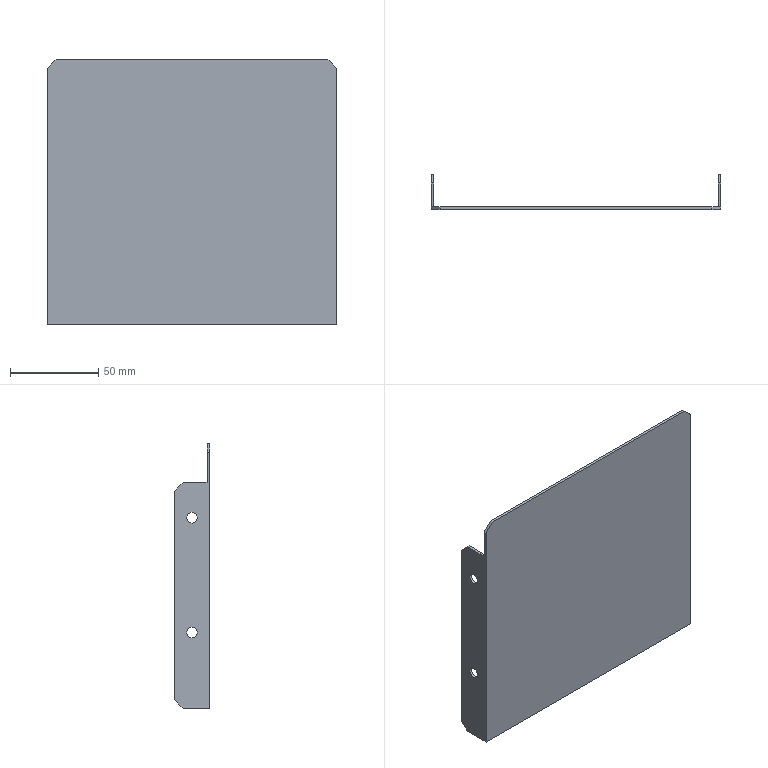Part | STEP file | MANG DAN PHOI BO GIUA | 1 solid | 26 faces | box 164 x 20 x 150 mm | volume 43722 mm3 | plane 18 | cylinder 8 | commonest cylinder face diameters 6 x8